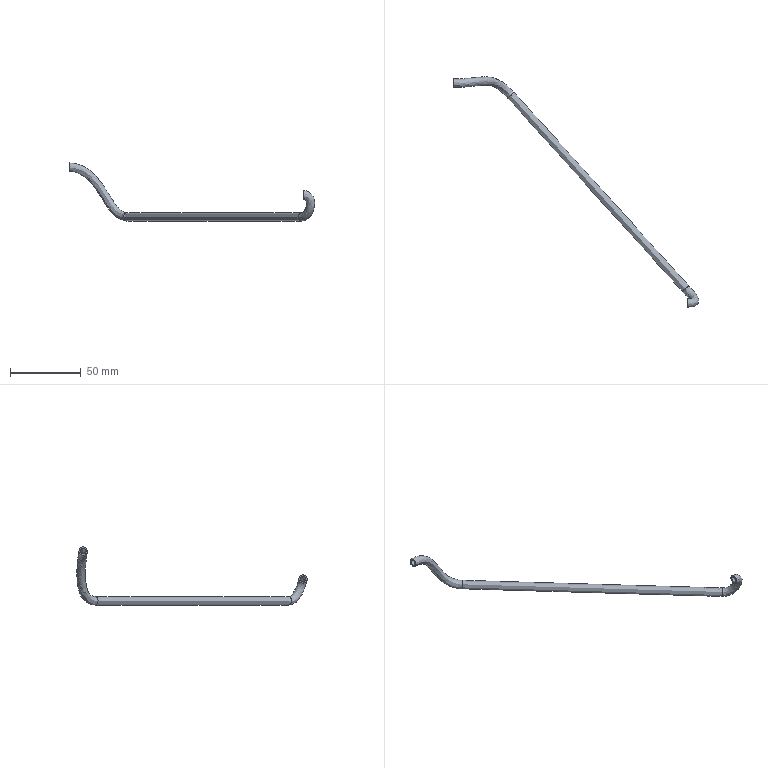Part | NX | features solid 2 | 1 solid | 8 faces | box 173.241 x 162.567 x 41.001 mm | volume 4008 mm3 | spline 6 | plane 2